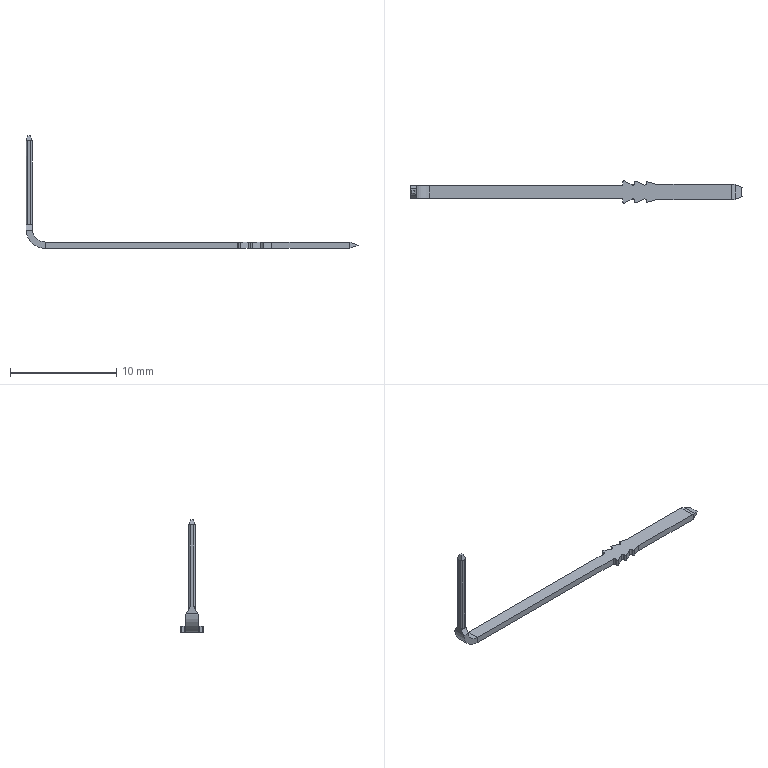Part | NX | features BREP 1 | 1 solid | 67 faces | box 31.2 x 2.1 x 10.6 mm | volume 27.788 mm3 | plane 36 | cylinder 31 | commonest cylinder face diameters 0.3 x12 0.2 x9 0.04 x4 0.025 x2 2 x2 2.4 x1